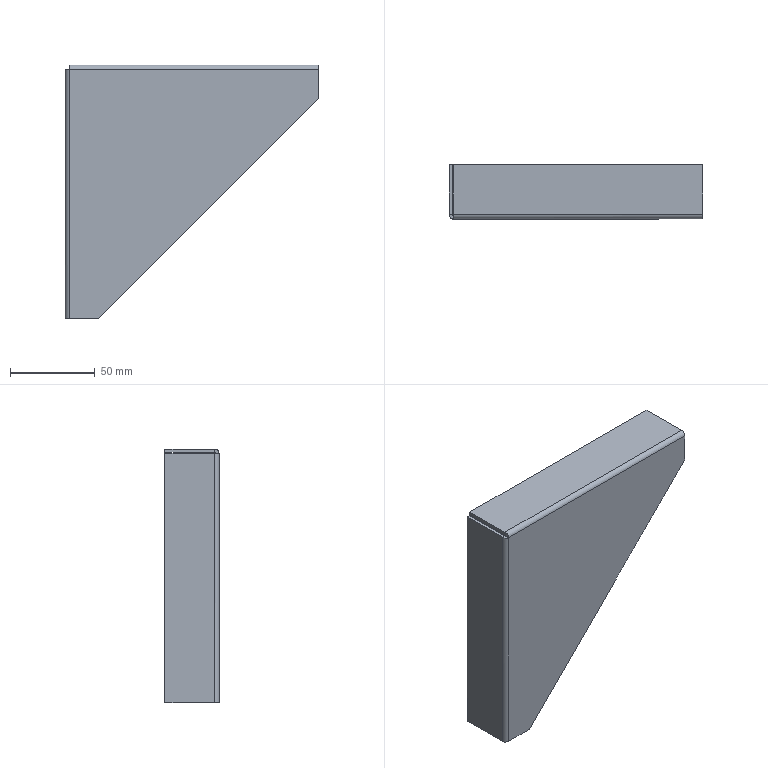Part | 1 solid | 19 faces | box 150 x 32 x 150 mm | volume 45364 mm3 | plane 13 | cylinder 4 | spline 2 | commonest cylinder face diameters 1.48 x2 5.48 x2
STEP:
#1=CARTESIAN_POINT('',(20.,-2.,-150.));
#2=VERTEX_POINT('',#1);
#3=CARTESIAN_POINT('',(2.74,-2.,-150.));
#4=VERTEX_POINT('',#3);
#5=CARTESIAN_POINT('',(0.,-2.,-150.));
#6=DIRECTION('',(-1.,0.,0.));
#7=VECTOR('',#6,1000.);
#8=LINE('',#5,#7);
#9=EDGE_CURVE('',#2,#4,#8,.T.);
#10=ORIENTED_EDGE('',*,*,#9,.T.);
#11=CARTESIAN_POINT('',(0.,0.74,-150.));
#12=VERTEX_POINT('',#11);
#13=CARTESIAN_POINT('',(2.74,0.74,-150.));
#14=DIRECTION('',(0.,0.,-1.));
#15=DIRECTION('',(-1.,0.,0.));
#16=AXIS2_PLACEMENT_3D('',#13,#14,#15);
#17=CIRCLE('',#16,2.74);
#18=EDGE_CURVE('',#4,#12,#17,.T.);
#19=ORIENTED_EDGE('',*,*,#18,.T.);
#20=CARTESIAN_POINT('',(0.,30.,-150.));
#21=VERTEX_POINT('',#20);
#22=CARTESIAN_POINT('',(0.,30.,-150.));
#23=DIRECTION('',(0.,1.,0.));
#24=VECTOR('',#23,1000.);
#25=LINE('',#22,#24);
#26=EDGE_CURVE('',#12,#21,#25,.T.);
#27=ORIENTED_EDGE('',*,*,#26,.T.);
#28=CARTESIAN_POINT('',(2.,30.,-150.));
#29=VERTEX_POINT('',#28);
#30=CARTESIAN_POINT('',(0.,30.,-150.));
#31=DIRECTION('',(-1.,0.,0.));
#32=VECTOR('',#31,1000.);
#33=LINE('',#30,#32);
#34=EDGE_CURVE('',#29,#21,#33,.T.);
#35=ORIENTED_EDGE('',*,*,#34,.F.);
#36=CARTESIAN_POINT('',(2.,0.74,-150.));
#37=VERTEX_POINT('',#36);
#38=CARTESIAN_POINT('',(2.,0.,-150.));
#39=DIRECTION('',(0.,1.,0.));
#40=VECTOR('',#39,1000.);
#41=LINE('',#38,#40);
#42=EDGE_CURVE('',#37,#29,#41,.T.);
#43=ORIENTED_EDGE('',*,*,#42,.F.);
#44=CARTESIAN_POINT('',(2.74,0.,-150.));
#45=VERTEX_POINT('',#44);
#46=CARTESIAN_POINT('',(2.74,0.74,-150.));
#47=DIRECTION('',(0.,0.,1.));
#48=DIRECTION('',(-1.,0.,0.));
#49=AXIS2_PLACEMENT_3D('',#46,#47,#48);
#50=CIRCLE('',#49,0.74);
#51=EDGE_CURVE('',#37,#45,#50,.T.);
#52=ORIENTED_EDGE('',*,*,#51,.T.);
#53=CARTESIAN_POINT('',(20.,0.,-150.));
#54=VERTEX_POINT('',#53);
#55=CARTESIAN_POINT('',(0.,0.,-150.));
#56=DIRECTION('',(-1.,0.,0.));
#57=VECTOR('',#56,1000.);
#58=LINE('',#55,#57);
#59=EDGE_CURVE('',#54,#45,#58,.T.);
#60=ORIENTED_EDGE('',*,*,#59,.F.);
#61=CARTESIAN_POINT('',(20.,-2.,-150.));
#62=DIRECTION('',(0.,1.,0.));
#63=VECTOR('',#62,1000.);
#64=LINE('',#61,#63);
#65=EDGE_CURVE('',#2,#54,#64,.T.);
#66=ORIENTED_EDGE('',*,*,#65,.F.);
#67=EDGE_LOOP('',(#10,#19,#27,#35,#43,#52,#60,#66));
#68=FACE_OUTER_BOUND('',#67,.T.);
#69=CARTESIAN_POINT('',(0.,-2.,-150.));
#70=DIRECTION('',(0.,0.,-1.));
#71=DIRECTION('',(-1.,0.,0.));
#72=AXIS2_PLACEMENT_3D('',#69,#70,#71);
#73=PLANE('',#72);
#74=ADVANCED_FACE('',(#68),#73,.T.);
#75=ORIENTED_EDGE('',*,*,#26,.F.);
#76=CARTESIAN_POINT('',(0.,0.74,-2.354));
#77=VERTEX_POINT('',#76);
#78=CARTESIAN_POINT('',(0.,0.74,0.));
#79=DIRECTION('',(0.,0.,1.));
#80=VECTOR('',#79,1000.);
#81=LINE('',#78,#80);
#82=EDGE_CURVE('',#12,#77,#81,.T.);
#83=ORIENTED_EDGE('',*,*,#82,.T.);
#84=CARTESIAN_POINT('',(0.,30.,-2.354));
#85=VERTEX_POINT('',#84);
#86=CARTESIAN_POINT('',(0.,30.,-2.354));
#87=DIRECTION('',(0.,-1.,0.));
#88=VECTOR('',#87,1000.);
#89=LINE('',#86,#88);
#90=EDGE_CURVE('',#85,#77,#89,.T.);
#91=ORIENTED_EDGE('',*,*,#90,.F.);
#92=CARTESIAN_POINT('',(0.,30.,-2.354));
#93=DIRECTION('',(0.,0.,1.));
#94=VECTOR('',#93,1000.);
#95=LINE('',#92,#94);
#96=EDGE_CURVE('',#21,#85,#95,.T.);
#97=ORIENTED_EDGE('',*,*,#96,.F.);
#98=EDGE_LOOP('',(#75,#83,#91,#97));
#99=FACE_OUTER_BOUND('',#98,.T.);
#100=CARTESIAN_POINT('',(0.,0.,0.));
#101=DIRECTION('',(-1.,0.,0.));
#102=DIRECTION('',(0.,-1.,0.));
#103=AXIS2_PLACEMENT_3D('',#100,#101,#102);
#104=PLANE('',#103);
#105=ADVANCED_FACE('',(#99),#104,.T.);
#106=CARTESIAN_POINT('',(2.,30.,-2.354));
#107=VERTEX_POINT('',#106);
#108=CARTESIAN_POINT('',(2.,0.74,-2.354));
#109=VERTEX_POINT('',#108);
#110=CARTESIAN_POINT('',(2.,30.,-2.354));
#111=DIRECTION('',(0.,-1.,0.));
#112=VECTOR('',#111,1000.);
#113=LINE('',#110,#112);
#114=EDGE_CURVE('',#107,#109,#113,.T.);
#115=ORIENTED_EDGE('',*,*,#114,.T.);
#116=CARTESIAN_POINT('',(2.,0.74,-150.));
#117=DIRECTION('',(0.,0.,-1.));
#118=VECTOR('',#117,1000.);
#119=LINE('',#116,#118);
#120=EDGE_CURVE('',#109,#37,#119,.T.);
#121=ORIENTED_EDGE('',*,*,#120,.T.);
#122=ORIENTED_EDGE('',*,*,#42,.T.);
#123=CARTESIAN_POINT('',(2.,30.,-150.));
#124=DIRECTION('',(0.,0.,-1.));
#125=VECTOR('',#124,1000.);
#126=LINE('',#123,#125);
#127=EDGE_CURVE('',#107,#29,#126,.T.);
#128=ORIENTED_EDGE('',*,*,#127,.F.);
#129=EDGE_LOOP('',(#115,#121,#122,#128));
#130=FACE_OUTER_BOUND('',#129,.T.);
#131=CARTESIAN_POINT('',(2.,0.,0.));
#132=DIRECTION('',(-1.,0.,0.));
#133=DIRECTION('',(0.,-1.,0.));
#134=AXIS2_PLACEMENT_3D('',#131,#132,#133);
#135=PLANE('',#134);
#136=ADVANCED_FACE('',(#130),#135,.F.);
#137=CARTESIAN_POINT('',(150.,30.,0.));
#138=VERTEX_POINT('',#137);
#139=CARTESIAN_POINT('',(150.,0.74,0.));
#140=VERTEX_POINT('',#139);
#141=CARTESIAN_POINT('',(150.,30.,0.));
#142=DIRECTION('',(0.,-1.,0.));
#143=VECTOR('',#142,1000.);
#144=LINE('',#141,#143);
#145=EDGE_CURVE('',#138,#140,#144,.T.);
#146=ORIENTED_EDGE('',*,*,#145,.T.);
#147=CARTESIAN_POINT('',(150.,-2.,-2.74));
#148=VERTEX_POINT('',#147);
#149=CARTESIAN_POINT('',(150.,0.74,-2.74));
#150=DIRECTION('',(1.,0.,0.));
#151=DIRECTION('',(0.,0.,-1.));
#152=AXIS2_PLACEMENT_3D('',#149,#150,#151);
#153=CIRCLE('',#152,2.74);
#154=EDGE_CURVE('',#140,#148,#153,.T.);
#155=ORIENTED_EDGE('',*,*,#154,.T.);
#156=CARTESIAN_POINT('',(150.,-2.,-20.));
#157=VERTEX_POINT('',#156);
#158=CARTESIAN_POINT('',(150.,-2.,-20.));
#159=DIRECTION('',(0.,0.,-1.));
#160=VECTOR('',#159,1000.);
#161=LINE('',#158,#160);
#162=EDGE_CURVE('',#148,#157,#161,.T.);
#163=ORIENTED_EDGE('',*,*,#162,.T.);
#164=CARTESIAN_POINT('',(150.,0.,-20.));
#165=VERTEX_POINT('',#164);
#166=CARTESIAN_POINT('',(150.,-2.,-20.));
#167=DIRECTION('',(0.,1.,0.));
#168=VECTOR('',#167,1000.);
#169=LINE('',#166,#168);
#170=EDGE_CURVE('',#157,#165,#169,.T.);
#171=ORIENTED_EDGE('',*,*,#170,.T.);
#172=CARTESIAN_POINT('',(150.,0.,-2.74));
#173=VERTEX_POINT('',#172);
#174=CARTESIAN_POINT('',(150.,0.,-20.));
#175=DIRECTION('',(0.,0.,-1.));
#176=VECTOR('',#175,1000.);
#177=LINE('',#174,#176);
#178=EDGE_CURVE('',#173,#165,#177,.T.);
#179=ORIENTED_EDGE('',*,*,#178,.F.);
#180=CARTESIAN_POINT('',(150.,0.74,-2.));
#181=VERTEX_POINT('',#180);
#182=CARTESIAN_POINT('',(150.,0.74,-2.74));
#183=DIRECTION('',(-1.,0.,0.));
#184=DIRECTION('',(0.,0.,-1.));
#185=AXIS2_PLACEMENT_3D('',#182,#183,#184);
#186=CIRCLE('',#185,0.74);
#187=EDGE_CURVE('',#173,#181,#186,.T.);
#188=ORIENTED_EDGE('',*,*,#187,.T.);
#189=CARTESIAN_POINT('',(150.,30.,-2.));
#190=VERTEX_POINT('',#189);
#191=CARTESIAN_POINT('',(150.,0.,-2.));
#192=DIRECTION('',(0.,-1.,0.));
#193=VECTOR('',#192,1000.);
#194=LINE('',#191,#193);
#195=EDGE_CURVE('',#190,#181,#194,.T.);
#196=ORIENTED_EDGE('',*,*,#195,.F.);
#197=CARTESIAN_POINT('',(150.,30.,-2.));
#198=DIRECTION('',(0.,0.,-1.));
#199=VECTOR('',#198,1000.);
#200=LINE('',#197,#199);
#201=EDGE_CURVE('',#138,#190,#200,.T.);
#202=ORIENTED_EDGE('',*,*,#201,.F.);
#203=EDGE_LOOP('',(#146,#155,#163,#171,#179,#188,#196,#202));
#204=FACE_OUTER_BOUND('',#203,.T.);
#205=CARTESIAN_POINT('',(150.,-2.,-20.));
#206=DIRECTION('',(1.,0.,0.));
#207=DIRECTION('',(0.,0.,-1.));
#208=AXIS2_PLACEMENT_3D('',#205,#206,#207);
#209=PLANE('',#208);
#210=ADVANCED_FACE('',(#204),#209,.T.);
#211=CARTESIAN_POINT('',(2.354,30.,0.));
#212=VERTEX_POINT('',#211);
#213=CARTESIAN_POINT('',(2.354,0.74,0.));
#214=VERTEX_POINT('',#213);
#215=CARTESIAN_POINT('',(2.354,30.,0.));
#216=DIRECTION('',(0.,-1.,0.));
#217=VECTOR('',#216,1000.);
#218=LINE('',#215,#217);
#219=EDGE_CURVE('',#212,#214,#218,.T.);
#220=ORIENTED_EDGE('',*,*,#219,.T.);
#221=CARTESIAN_POINT('',(150.,0.74,0.));
#222=DIRECTION('',(1.,0.,0.));
#223=VECTOR('',#222,1000.);
#224=LINE('',#221,#223);
#225=EDGE_CURVE('',#214,#140,#224,.T.);
#226=ORIENTED_EDGE('',*,*,#225,.T.);
#227=ORIENTED_EDGE('',*,*,#145,.F.);
#228=CARTESIAN_POINT('',(150.,30.,0.));
#229=DIRECTION('',(1.,0.,0.));
#230=VECTOR('',#229,1000.);
#231=LINE('',#228,#230);
#232=EDGE_CURVE('',#212,#138,#231,.T.);
#233=ORIENTED_EDGE('',*,*,#232,.F.);
#234=EDGE_LOOP('',(#220,#226,#227,#233));
#235=FACE_OUTER_BOUND('',#234,.T.);
#236=CARTESIAN_POINT('',(0.,0.,0.));
#237=DIRECTION('',(0.,0.,-1.));
#238=DIRECTION('',(0.,1.,0.));
#239=AXIS2_PLACEMENT_3D('',#236,#237,#238);
#240=PLANE('',#239);
#241=ADVANCED_FACE('',(#235),#240,.F.);
#242=ORIENTED_EDGE('',*,*,#195,.T.);
#243=CARTESIAN_POINT('',(2.354,0.74,-2.));
#244=VERTEX_POINT('',#243);
#245=CARTESIAN_POINT('',(0.,0.74,-2.));
#246=DIRECTION('',(-1.,0.,0.));
#247=VECTOR('',#246,1000.);
#248=LINE('',#245,#247);
#249=EDGE_CURVE('',#181,#244,#248,.T.);
#250=ORIENTED_EDGE('',*,*,#249,.T.);
#251=CARTESIAN_POINT('',(2.354,30.,-2.));
#252=VERTEX_POINT('',#251);
#253=CARTESIAN_POINT('',(2.354,30.,-2.));
#254=DIRECTION('',(0.,-1.,0.));
#255=VECTOR('',#254,1000.);
#256=LINE('',#253,#255);
#257=EDGE_CURVE('',#252,#244,#256,.T.);
#258=ORIENTED_EDGE('',*,*,#257,.F.);
#259=CARTESIAN_POINT('',(2.354,30.,-2.));
#260=DIRECTION('',(-1.,0.,0.));
#261=VECTOR('',#260,1000.);
#262=LINE('',#259,#261);
#263=EDGE_CURVE('',#190,#252,#262,.T.);
#264=ORIENTED_EDGE('',*,*,#263,.F.);
#265=EDGE_LOOP('',(#242,#250,#258,#264));
#266=FACE_OUTER_BOUND('',#265,.T.);
#267=CARTESIAN_POINT('',(0.,0.,-2.));
#268=DIRECTION('',(0.,0.,-1.));
#269=DIRECTION('',(0.,1.,0.));
#270=AXIS2_PLACEMENT_3D('',#267,#268,#269);
#271=PLANE('',#270);
#272=ADVANCED_FACE('',(#266),#271,.T.);
#273=ORIENTED_EDGE('',*,*,#162,.F.);
#274=CARTESIAN_POINT('',(2.74,-2.,-2.74));
#275=VERTEX_POINT('',#274);
#276=CARTESIAN_POINT('',(2.547,-2.,-2.74));
#277=DIRECTION('',(-1.,0.,0.));
#278=VECTOR('',#277,1000.);
#279=LINE('',#276,#278);
#280=EDGE_CURVE('',#148,#275,#279,.T.);
#281=ORIENTED_EDGE('',*,*,#280,.T.);
#282=CARTESIAN_POINT('',(2.74,-2.,0.));
#283=DIRECTION('',(0.,0.,-1.));
#284=VECTOR('',#283,1000.);
#285=LINE('',#282,#284);
#286=EDGE_CURVE('',#275,#4,#285,.T.);
#287=ORIENTED_EDGE('',*,*,#286,.T.);
#288=ORIENTED_EDGE('',*,*,#9,.F.);
#289=CARTESIAN_POINT('',(20.,-2.,-150.));
#290=DIRECTION('',(-0.7071,0.,-0.7071));
#291=VECTOR('',#290,1000.);
#292=LINE('',#289,#291);
#293=EDGE_CURVE('',#157,#2,#292,.T.);
#294=ORIENTED_EDGE('',*,*,#293,.F.);
#295=EDGE_LOOP('',(#273,#281,#287,#288,#294));
#296=FACE_OUTER_BOUND('',#295,.T.);
#297=CARTESIAN_POINT('',(0.,-2.,0.));
#298=DIRECTION('',(0.,-1.,0.));
#299=DIRECTION('',(0.,0.,-1.));
#300=AXIS2_PLACEMENT_3D('',#297,#298,#299);
#301=PLANE('',#300);
#302=ADVANCED_FACE('',(#296),#301,.T.);
#303=CARTESIAN_POINT('',(2.74,0.,-2.74));
#304=VERTEX_POINT('',#303);
#305=CARTESIAN_POINT('',(2.74,0.,-2.547));
#306=DIRECTION('',(0.,0.,1.));
#307=VECTOR('',#306,1000.);
#308=LINE('',#305,#307);
#309=EDGE_CURVE('',#45,#304,#308,.T.);
#310=ORIENTED_EDGE('',*,*,#309,.T.);
#311=CARTESIAN_POINT('',(0.,0.,-2.74));
#312=DIRECTION('',(1.,0.,0.));
#313=VECTOR('',#312,1000.);
#314=LINE('',#311,#313);
#315=EDGE_CURVE('',#304,#173,#314,.T.);
#316=ORIENTED_EDGE('',*,*,#315,.T.);
#317=ORIENTED_EDGE('',*,*,#178,.T.);
#318=CARTESIAN_POINT('',(20.,0.,-150.));
#319=DIRECTION('',(-0.7071,0.,-0.7071));
#320=VECTOR('',#319,1000.);
#321=LINE('',#318,#320);
#322=EDGE_CURVE('',#165,#54,#321,.T.);
#323=ORIENTED_EDGE('',*,*,#322,.T.);
#324=ORIENTED_EDGE('',*,*,#59,.T.);
#325=EDGE_LOOP('',(#310,#316,#317,#323,#324));
#326=FACE_OUTER_BOUND('',#325,.T.);
#327=CARTESIAN_POINT('',(0.,0.,0.));
#328=DIRECTION('',(0.,-1.,0.));
#329=DIRECTION('',(0.,0.,-1.));
#330=AXIS2_PLACEMENT_3D('',#327,#328,#329);
#331=PLANE('',#330);
#332=ADVANCED_FACE('',(#326),#331,.F.);
#333=ORIENTED_EDGE('',*,*,#322,.F.);
#334=ORIENTED_EDGE('',*,*,#170,.F.);
#335=ORIENTED_EDGE('',*,*,#293,.T.);
#336=ORIENTED_EDGE('',*,*,#65,.T.);
#337=EDGE_LOOP('',(#333,#334,#335,#336));
#338=FACE_OUTER_BOUND('',#337,.T.);
#339=CARTESIAN_POINT('',(20.,-2.,-150.));
#340=DIRECTION('',(0.7071,0.,-0.7071));
#341=DIRECTION('',(-0.7071,0.,-0.7071));
#342=AXIS2_PLACEMENT_3D('',#339,#340,#341);
#343=PLANE('',#342);
#344=ADVANCED_FACE('',(#338),#343,.T.);
#345=CARTESIAN_POINT('',(2.,0.74,-2.354));
#346=DIRECTION('',(1.,0.,0.));
#347=VECTOR('',#346,1000.);
#348=LINE('',#345,#347);
#349=EDGE_CURVE('',#77,#109,#348,.T.);
#350=ORIENTED_EDGE('',*,*,#349,.F.);
#351=CARTESIAN_POINT('',(0.,0.74,-2.354));
#352=CARTESIAN_POINT('',(0.,0.5591,-2.37));
#353=CARTESIAN_POINT('',(0.01774,0.3812,-2.386));
#354=CARTESIAN_POINT('',(0.08726,0.03121,-2.418));
#355=CARTESIAN_POINT('',(0.1399,-0.1427,-2.434));
#356=CARTESIAN_POINT('',(0.2773,-0.4744,-2.466));
#357=CARTESIAN_POINT('',(0.3613,-0.6317,-2.482));
#358=CARTESIAN_POINT('',(0.5599,-0.9294,-2.514));
#359=CARTESIAN_POINT('',(0.6755,-1.07,-2.531));
#360=CARTESIAN_POINT('',(0.9281,-1.323,-2.563));
#361=CARTESIAN_POINT('',(1.066,-1.437,-2.579));
#362=CARTESIAN_POINT('',(1.365,-1.637,-2.611));
#363=CARTESIAN_POINT('',(1.525,-1.722,-2.627));
#364=CARTESIAN_POINT('',(2.019,-1.927,-2.675));
#365=CARTESIAN_POINT('',(2.378,-2.,-2.708));
#366=CARTESIAN_POINT('',(2.74,-2.,-2.74));
#367=B_SPLINE_CURVE_WITH_KNOTS('',3,(#351,#352,#353,#354,#355,#356,#357,#358,#359,#360,#361,#362,#363,#364,#365,#366),.UNSPECIFIED.,.F.,.F.,(4,2,2,2,2,2,2,4),(0.,0.0005372,0.001074,0.001612,0.002149,0.002686,0.003223,0.004297),.UNSPECIFIED.);
#368=EDGE_CURVE('',#77,#275,#367,.T.);
#369=ORIENTED_EDGE('',*,*,#368,.T.);
#370=CARTESIAN_POINT('',(2.74,0.,-2.74));
#371=DIRECTION('',(0.,-1.,0.));
#372=VECTOR('',#371,1000.);
#373=LINE('',#370,#372);
#374=EDGE_CURVE('',#304,#275,#373,.T.);
#375=ORIENTED_EDGE('',*,*,#374,.F.);
#376=CARTESIAN_POINT('',(2.74,0.,-2.74));
#377=CARTESIAN_POINT('',(2.642,0.,-2.708));
#378=CARTESIAN_POINT('',(2.547,0.01912,-2.676));
#379=CARTESIAN_POINT('',(2.367,0.09351,-2.611));
#380=CARTESIAN_POINT('',(2.285,0.1482,-2.579));
#381=CARTESIAN_POINT('',(2.08,0.3535,-2.482));
#382=CARTESIAN_POINT('',(2.,0.5446,-2.419));
#383=CARTESIAN_POINT('',(2.,0.74,-2.354));
#384=B_SPLINE_CURVE_WITH_KNOTS('',3,(#376,#377,#378,#379,#380,#381,#382,#383),.UNSPECIFIED.,.F.,.F.,(4,2,2,4),(0.,0.0003046,0.0006091,0.001218),.UNSPECIFIED.);
#385=EDGE_CURVE('',#304,#109,#384,.T.);
#386=ORIENTED_EDGE('',*,*,#385,.T.);
#387=EDGE_LOOP('',(#350,#369,#375,#386));
#388=FACE_OUTER_BOUND('',#387,.T.);
#389=CARTESIAN_POINT('',(-1.154,0.74,-2.354));
#390=CARTESIAN_POINT('',(-1.154,0.2302,-2.386));
#391=CARTESIAN_POINT('',(-1.052,-0.2792,-2.418));
#392=CARTESIAN_POINT('',(-0.6623,-1.221,-2.482));
#393=CARTESIAN_POINT('',(-0.3737,-1.653,-2.515));
#394=CARTESIAN_POINT('',(0.3471,-2.374,-2.579));
#395=CARTESIAN_POINT('',(0.779,-2.662,-2.611));
#396=CARTESIAN_POINT('',(1.721,-3.052,-2.676));
#397=CARTESIAN_POINT('',(2.23,-3.154,-2.708));
#398=CARTESIAN_POINT('',(2.74,-3.154,-2.74));
#399=CARTESIAN_POINT('',(-0.02,0.74,-2.354));
#400=CARTESIAN_POINT('',(-0.02,0.3787,-2.386));
#401=CARTESIAN_POINT('',(0.05184,0.01758,-2.418));
#402=CARTESIAN_POINT('',(0.3283,-0.65,-2.482));
#403=CARTESIAN_POINT('',(0.5329,-0.9561,-2.515));
#404=CARTESIAN_POINT('',(1.044,-1.467,-2.579));
#405=CARTESIAN_POINT('',(1.35,-1.672,-2.611));
#406=CARTESIAN_POINT('',(2.018,-1.948,-2.676));
#407=CARTESIAN_POINT('',(2.379,-2.02,-2.708));
#408=CARTESIAN_POINT('',(2.74,-2.02,-2.74));
#409=CARTESIAN_POINT('',(0.,0.74,-2.354));
#410=CARTESIAN_POINT('',(0.,0.3813,-2.386));
#411=CARTESIAN_POINT('',(0.07131,0.02281,-2.418));
#412=CARTESIAN_POINT('',(0.3458,-0.6399,-2.482));
#413=CARTESIAN_POINT('',(0.5489,-0.9439,-2.515));
#414=CARTESIAN_POINT('',(1.056,-1.451,-2.579));
#415=CARTESIAN_POINT('',(1.36,-1.654,-2.611));
#416=CARTESIAN_POINT('',(2.023,-1.929,-2.676));
#417=CARTESIAN_POINT('',(2.381,-2.,-2.708));
#418=CARTESIAN_POINT('',(2.74,-2.,-2.74));
#419=CARTESIAN_POINT('',(2.,0.74,-2.354));
#420=CARTESIAN_POINT('',(2.,0.6431,-2.386));
#421=CARTESIAN_POINT('',(2.019,0.5463,-2.418));
#422=CARTESIAN_POINT('',(2.093,0.3673,-2.482));
#423=CARTESIAN_POINT('',(2.148,0.2852,-2.515));
#424=CARTESIAN_POINT('',(2.285,0.1482,-2.579));
#425=CARTESIAN_POINT('',(2.367,0.0934,-2.611));
#426=CARTESIAN_POINT('',(2.546,0.01926,-2.676));
#427=CARTESIAN_POINT('',(2.643,0.,-2.708));
#428=CARTESIAN_POINT('',(2.74,0.,-2.74));
#429=CARTESIAN_POINT('',(2.02,0.74,-2.354));
#430=CARTESIAN_POINT('',(2.02,0.6458,-2.386));
#431=CARTESIAN_POINT('',(2.039,0.5516,-2.418));
#432=CARTESIAN_POINT('',(2.111,0.3775,-2.482));
#433=CARTESIAN_POINT('',(2.164,0.2976,-2.515));
#434=CARTESIAN_POINT('',(2.298,0.1644,-2.579));
#435=CARTESIAN_POINT('',(2.377,0.111,-2.611));
#436=CARTESIAN_POINT('',(2.552,0.03893,-2.676));
#437=CARTESIAN_POINT('',(2.646,0.0202,-2.708));
#438=CARTESIAN_POINT('',(2.74,0.0202,-2.74));
#439=B_SPLINE_SURFACE_WITH_KNOTS('',1,3,((#389,#390,#391,#392,#393,#394,#395,#396,#397,#398),(#399,#400,#401,#402,#403,#404,#405,#406,#407,#408),(#409,#410,#411,#412,#413,#414,#415,#416,#417,#418),(#419,#420,#421,#422,#423,#424,#425,#426,#427,#428),(#429,#430,#431,#432,#433,#434,#435,#436,#437,#438)),.UNSPECIFIED.,.F.,.F.,.F.,(2,1,1,1,2),(4,2,2,2,4),(-0.5769,-0.01,0.,1.,1.01),(0.,0.25,0.5,0.75,1.),.UNSPECIFIED.);
#440=ADVANCED_FACE('',(#388),#439,.F.);
#441=ORIENTED_EDGE('',*,*,#374,.T.);
#442=CARTESIAN_POINT('',(2.74,-2.,-2.74));
#443=CARTESIAN_POINT('',(2.724,-2.,-2.559));
#444=CARTESIAN_POINT('',(2.708,-1.982,-2.381));
#445=CARTESIAN_POINT('',(2.676,-1.913,-2.031));
#446=CARTESIAN_POINT('',(2.66,-1.86,-1.857));
#447=CARTESIAN_POINT('',(2.627,-1.723,-1.526));
#448=CARTESIAN_POINT('',(2.611,-1.639,-1.368));
#449=CARTESIAN_POINT('',(2.579,-1.44,-1.071));
#450=CARTESIAN_POINT('',(2.563,-1.324,-0.9296));
#451=CARTESIAN_POINT('',(2.531,-1.072,-0.6768));
#452=CARTESIAN_POINT('',(2.515,-0.9341,-0.5634));
#453=CARTESIAN_POINT('',(2.483,-0.635,-0.3632));
#454=CARTESIAN_POINT('',(2.466,-0.4755,-0.2779));
#455=CARTESIAN_POINT('',(2.418,0.01865,-0.0727));
#456=CARTESIAN_POINT('',(2.386,0.3782,0.));
#457=CARTESIAN_POINT('',(2.354,0.74,0.));
#458=B_SPLINE_CURVE_WITH_KNOTS('',3,(#442,#443,#444,#445,#446,#447,#448,#449,#450,#451,#452,#453,#454,#455,#456,#457),.UNSPECIFIED.,.F.,.F.,(4,2,2,2,2,2,2,4),(0.,0.0005372,0.001074,0.001612,0.002149,0.002686,0.003223,0.004297),.UNSPECIFIED.);
#459=EDGE_CURVE('',#275,#214,#458,.T.);
#460=ORIENTED_EDGE('',*,*,#459,.T.);
#461=CARTESIAN_POINT('',(2.354,0.74,-2.));
#462=DIRECTION('',(0.,0.,-1.));
#463=VECTOR('',#462,1000.);
#464=LINE('',#461,#463);
#465=EDGE_CURVE('',#214,#244,#464,.T.);
#466=ORIENTED_EDGE('',*,*,#465,.T.);
#467=CARTESIAN_POINT('',(2.354,0.74,-2.));
#468=CARTESIAN_POINT('',(2.386,0.6423,-2.));
#469=CARTESIAN_POINT('',(2.418,0.5466,-2.019));
#470=CARTESIAN_POINT('',(2.482,0.367,-2.094));
#471=CARTESIAN_POINT('',(2.515,0.2853,-2.148));
#472=CARTESIAN_POINT('',(2.611,0.07993,-2.353));
#473=CARTESIAN_POINT('',(2.675,0.,-2.545));
#474=CARTESIAN_POINT('',(2.74,0.,-2.74));
#475=B_SPLINE_CURVE_WITH_KNOTS('',3,(#467,#468,#469,#470,#471,#472,#473,#474),.UNSPECIFIED.,.F.,.F.,(4,2,2,4),(0.,0.0003046,0.0006091,0.001218),.UNSPECIFIED.);
#476=EDGE_CURVE('',#244,#304,#475,.T.);
#477=ORIENTED_EDGE('',*,*,#476,.T.);
#478=EDGE_LOOP('',(#441,#460,#466,#477));
#479=FACE_OUTER_BOUND('',#478,.T.);
#480=CARTESIAN_POINT('',(2.74,-3.154,-2.74));
#481=CARTESIAN_POINT('',(2.708,-3.154,-2.23));
#482=CARTESIAN_POINT('',(2.676,-3.052,-1.721));
#483=CARTESIAN_POINT('',(2.611,-2.662,-0.779));
#484=CARTESIAN_POINT('',(2.579,-2.374,-0.3471));
#485=CARTESIAN_POINT('',(2.515,-1.653,0.3737));
#486=CARTESIAN_POINT('',(2.482,-1.221,0.6623));
#487=CARTESIAN_POINT('',(2.418,-0.2792,1.052));
#488=CARTESIAN_POINT('',(2.386,0.2302,1.154));
#489=CARTESIAN_POINT('',(2.354,0.74,1.154));
#490=CARTESIAN_POINT('',(2.74,-2.02,-2.74));
#491=CARTESIAN_POINT('',(2.708,-2.02,-2.379));
#492=CARTESIAN_POINT('',(2.676,-1.948,-2.018));
#493=CARTESIAN_POINT('',(2.611,-1.672,-1.35));
#494=CARTESIAN_POINT('',(2.579,-1.467,-1.044));
#495=CARTESIAN_POINT('',(2.515,-0.9561,-0.5329));
#496=CARTESIAN_POINT('',(2.482,-0.65,-0.3283));
#497=CARTESIAN_POINT('',(2.418,0.01758,-0.05184));
#498=CARTESIAN_POINT('',(2.386,0.3787,0.02));
#499=CARTESIAN_POINT('',(2.354,0.74,0.02));
#500=CARTESIAN_POINT('',(2.74,-2.,-2.74));
#501=CARTESIAN_POINT('',(2.708,-2.,-2.381));
#502=CARTESIAN_POINT('',(2.676,-1.929,-2.023));
#503=CARTESIAN_POINT('',(2.611,-1.654,-1.36));
#504=CARTESIAN_POINT('',(2.579,-1.451,-1.056));
#505=CARTESIAN_POINT('',(2.515,-0.9439,-0.5489));
#506=CARTESIAN_POINT('',(2.482,-0.6399,-0.3458));
#507=CARTESIAN_POINT('',(2.418,0.02281,-0.07131));
#508=CARTESIAN_POINT('',(2.386,0.3813,0.));
#509=CARTESIAN_POINT('',(2.354,0.74,0.));
#510=CARTESIAN_POINT('',(2.74,0.,-2.74));
#511=CARTESIAN_POINT('',(2.708,0.,-2.643));
#512=CARTESIAN_POINT('',(2.676,0.01926,-2.546));
#513=CARTESIAN_POINT('',(2.611,0.0934,-2.367));
#514=CARTESIAN_POINT('',(2.579,0.1482,-2.285));
#515=CARTESIAN_POINT('',(2.515,0.2852,-2.148));
#516=CARTESIAN_POINT('',(2.482,0.3673,-2.093));
#517=CARTESIAN_POINT('',(2.418,0.5463,-2.019));
#518=CARTESIAN_POINT('',(2.386,0.6431,-2.));
#519=CARTESIAN_POINT('',(2.354,0.74,-2.));
#520=CARTESIAN_POINT('',(2.74,0.0202,-2.74));
#521=CARTESIAN_POINT('',(2.708,0.0202,-2.646));
#522=CARTESIAN_POINT('',(2.676,0.03893,-2.552));
#523=CARTESIAN_POINT('',(2.611,0.111,-2.377));
#524=CARTESIAN_POINT('',(2.579,0.1644,-2.298));
#525=CARTESIAN_POINT('',(2.515,0.2976,-2.164));
#526=CARTESIAN_POINT('',(2.482,0.3775,-2.111));
#527=CARTESIAN_POINT('',(2.418,0.5516,-2.039));
#528=CARTESIAN_POINT('',(2.386,0.6458,-2.02));
#529=CARTESIAN_POINT('',(2.354,0.74,-2.02));
#530=B_SPLINE_SURFACE_WITH_KNOTS('',1,3,((#480,#481,#482,#483,#484,#485,#486,#487,#488,#489),(#490,#491,#492,#493,#494,#495,#496,#497,#498,#499),(#500,#501,#502,#503,#504,#505,#506,#507,#508,#509),(#510,#511,#512,#513,#514,#515,#516,#517,#518,#519),(#520,#521,#522,#523,#524,#525,#526,#527,#528,#529)),.UNSPECIFIED.,.F.,.F.,.F.,(2,1,1,1,2),(4,2,2,2,4),(-0.5769,-0.01,0.,1.,1.01),(0.,0.25,0.5,0.75,1.),.UNSPECIFIED.);
#531=ADVANCED_FACE('',(#479),#530,.F.);
#532=ORIENTED_EDGE('',*,*,#349,.T.);
#533=ORIENTED_EDGE('',*,*,#114,.F.);
#534=CARTESIAN_POINT('',(2.,30.,-2.354));
#535=DIRECTION('',(1.,0.,0.));
#536=VECTOR('',#535,1000.);
#537=LINE('',#534,#536);
#538=EDGE_CURVE('',#85,#107,#537,.T.);
#539=ORIENTED_EDGE('',*,*,#538,.F.);
#540=ORIENTED_EDGE('',*,*,#90,.T.);
#541=EDGE_LOOP('',(#532,#533,#539,#540));
#542=FACE_OUTER_BOUND('',#541,.T.);
#543=CARTESIAN_POINT('',(2.,30.,-2.354));
#544=DIRECTION('',(0.,0.,-1.));
#545=DIRECTION('',(-1.,0.,0.));
#546=AXIS2_PLACEMENT_3D('',#543,#544,#545);
#547=PLANE('',#546);
#548=ADVANCED_FACE('',(#542),#547,.F.);
#549=ORIENTED_EDGE('',*,*,#127,.T.);
#550=ORIENTED_EDGE('',*,*,#34,.T.);
#551=ORIENTED_EDGE('',*,*,#96,.T.);
#552=ORIENTED_EDGE('',*,*,#538,.T.);
#553=EDGE_LOOP('',(#549,#550,#551,#552));
#554=FACE_OUTER_BOUND('',#553,.T.);
#555=CARTESIAN_POINT('',(0.,30.,0.));
#556=DIRECTION('',(0.,-1.,0.));
#557=DIRECTION('',(1.,0.,0.));
#558=AXIS2_PLACEMENT_3D('',#555,#556,#557);
#559=PLANE('',#558);
#560=ADVANCED_FACE('',(#554),#559,.F.);
#561=ORIENTED_EDGE('',*,*,#465,.F.);
#562=ORIENTED_EDGE('',*,*,#219,.F.);
#563=CARTESIAN_POINT('',(2.354,30.,0.));
#564=DIRECTION('',(0.,0.,1.));
#565=VECTOR('',#564,1000.);
#566=LINE('',#563,#565);
#567=EDGE_CURVE('',#252,#212,#566,.T.);
#568=ORIENTED_EDGE('',*,*,#567,.F.);
#569=ORIENTED_EDGE('',*,*,#257,.T.);
#570=EDGE_LOOP('',(#561,#562,#568,#569));
#571=FACE_OUTER_BOUND('',#570,.T.);
#572=CARTESIAN_POINT('',(2.354,30.,0.));
#573=DIRECTION('',(1.,0.,0.));
#574=DIRECTION('',(0.,0.,-1.));
#575=AXIS2_PLACEMENT_3D('',#572,#573,#574);
#576=PLANE('',#575);
#577=ADVANCED_FACE('',(#571),#576,.F.);
#578=ORIENTED_EDGE('',*,*,#567,.T.);
#579=ORIENTED_EDGE('',*,*,#232,.T.);
#580=ORIENTED_EDGE('',*,*,#201,.T.);
#581=ORIENTED_EDGE('',*,*,#263,.T.);
#582=EDGE_LOOP('',(#578,#579,#580,#581));
#583=FACE_OUTER_BOUND('',#582,.T.);
#584=CARTESIAN_POINT('',(0.,30.,0.));
#585=DIRECTION('',(0.,-1.,0.));
#586=DIRECTION('',(0.,0.,-1.));
#587=AXIS2_PLACEMENT_3D('',#584,#585,#586);
#588=PLANE('',#587);
#589=ADVANCED_FACE('',(#583),#588,.F.);
#590=ORIENTED_EDGE('',*,*,#476,.F.);
#591=ORIENTED_EDGE('',*,*,#249,.F.);
#592=ORIENTED_EDGE('',*,*,#187,.F.);
#593=ORIENTED_EDGE('',*,*,#315,.F.);
#594=EDGE_LOOP('',(#590,#591,#592,#593));
#595=FACE_OUTER_BOUND('',#594,.T.);
#596=CARTESIAN_POINT('',(0.,0.74,-2.74));
#597=DIRECTION('',(1.,0.,0.));
#598=DIRECTION('',(0.,0.,-1.));
#599=AXIS2_PLACEMENT_3D('',#596,#597,#598);
#600=CYLINDRICAL_SURFACE('',#599,0.74);
#601=ADVANCED_FACE('',(#595),#600,.F.);
#602=ORIENTED_EDGE('',*,*,#51,.F.);
#603=ORIENTED_EDGE('',*,*,#120,.F.);
#604=ORIENTED_EDGE('',*,*,#385,.F.);
#605=ORIENTED_EDGE('',*,*,#309,.F.);
#606=EDGE_LOOP('',(#602,#603,#604,#605));
#607=FACE_OUTER_BOUND('',#606,.T.);
#608=CARTESIAN_POINT('',(2.74,0.74,0.));
#609=DIRECTION('',(0.,0.,-1.));
#610=DIRECTION('',(-1.,0.,0.));
#611=AXIS2_PLACEMENT_3D('',#608,#609,#610);
#612=CYLINDRICAL_SURFACE('',#611,0.74);
#613=ADVANCED_FACE('',(#607),#612,.F.);
#614=ORIENTED_EDGE('',*,*,#154,.F.);
#615=ORIENTED_EDGE('',*,*,#225,.F.);
#616=ORIENTED_EDGE('',*,*,#459,.F.);
#617=ORIENTED_EDGE('',*,*,#280,.F.);
#618=EDGE_LOOP('',(#614,#615,#616,#617));
#619=FACE_OUTER_BOUND('',#618,.T.);
#620=CARTESIAN_POINT('',(0.,0.74,-2.74));
#621=DIRECTION('',(1.,0.,0.));
#622=DIRECTION('',(0.,0.,-1.));
#623=AXIS2_PLACEMENT_3D('',#620,#621,#622);
#624=CYLINDRICAL_SURFACE('',#623,2.74);
#625=ADVANCED_FACE('',(#619),#624,.T.);
#626=ORIENTED_EDGE('',*,*,#18,.F.);
#627=ORIENTED_EDGE('',*,*,#286,.F.);
#628=ORIENTED_EDGE('',*,*,#368,.F.);
#629=ORIENTED_EDGE('',*,*,#82,.F.);
#630=EDGE_LOOP('',(#626,#627,#628,#629));
#631=FACE_OUTER_BOUND('',#630,.T.);
#632=CARTESIAN_POINT('',(2.74,0.74,0.));
#633=DIRECTION('',(0.,0.,1.));
#634=DIRECTION('',(1.,0.,0.));
#635=AXIS2_PLACEMENT_3D('',#632,#633,#634);
#636=CYLINDRICAL_SURFACE('',#635,2.74);
#637=ADVANCED_FACE('',(#631),#636,.T.);
#638=CLOSED_SHELL('',(#74,#105,#136,#210,#241,#272,#302,#332,#344,#440,#531,#548,#560,#577,#589,#601,#613,#625,#637));
#639=MANIFOLD_SOLID_BREP('',#638);
#640=CARTESIAN_POINT('',(0.,0.,0.));
#641=DIRECTION('',(0.,0.,1.));
#642=DIRECTION('',(1.,0.,0.));
#643=AXIS2_PLACEMENT_3D('',#640,#641,#642);
#644=(LENGTH_UNIT()NAMED_UNIT(*)SI_UNIT(.MILLI.,.METRE.));
#645=UNCERTAINTY_MEASURE_WITH_UNIT(LENGTH_MEASURE(0.00001),#644,'','');
#646=(NAMED_UNIT(*)PLANE_ANGLE_UNIT()SI_UNIT($,.RADIAN.));
#647=(NAMED_UNIT(*)SI_UNIT($,.STERADIAN.)SOLID_ANGLE_UNIT());
#648=(GEOMETRIC_REPRESENTATION_CONTEXT(3)GLOBAL_UNCERTAINTY_ASSIGNED_CONTEXT((#645))GLOBAL_UNIT_ASSIGNED_CONTEXT((#644,#646,#647))REPRESENTATION_CONTEXT('',''));
#649=ADVANCED_BREP_SHAPE_REPRESENTATION('',(#639,#643),#648);